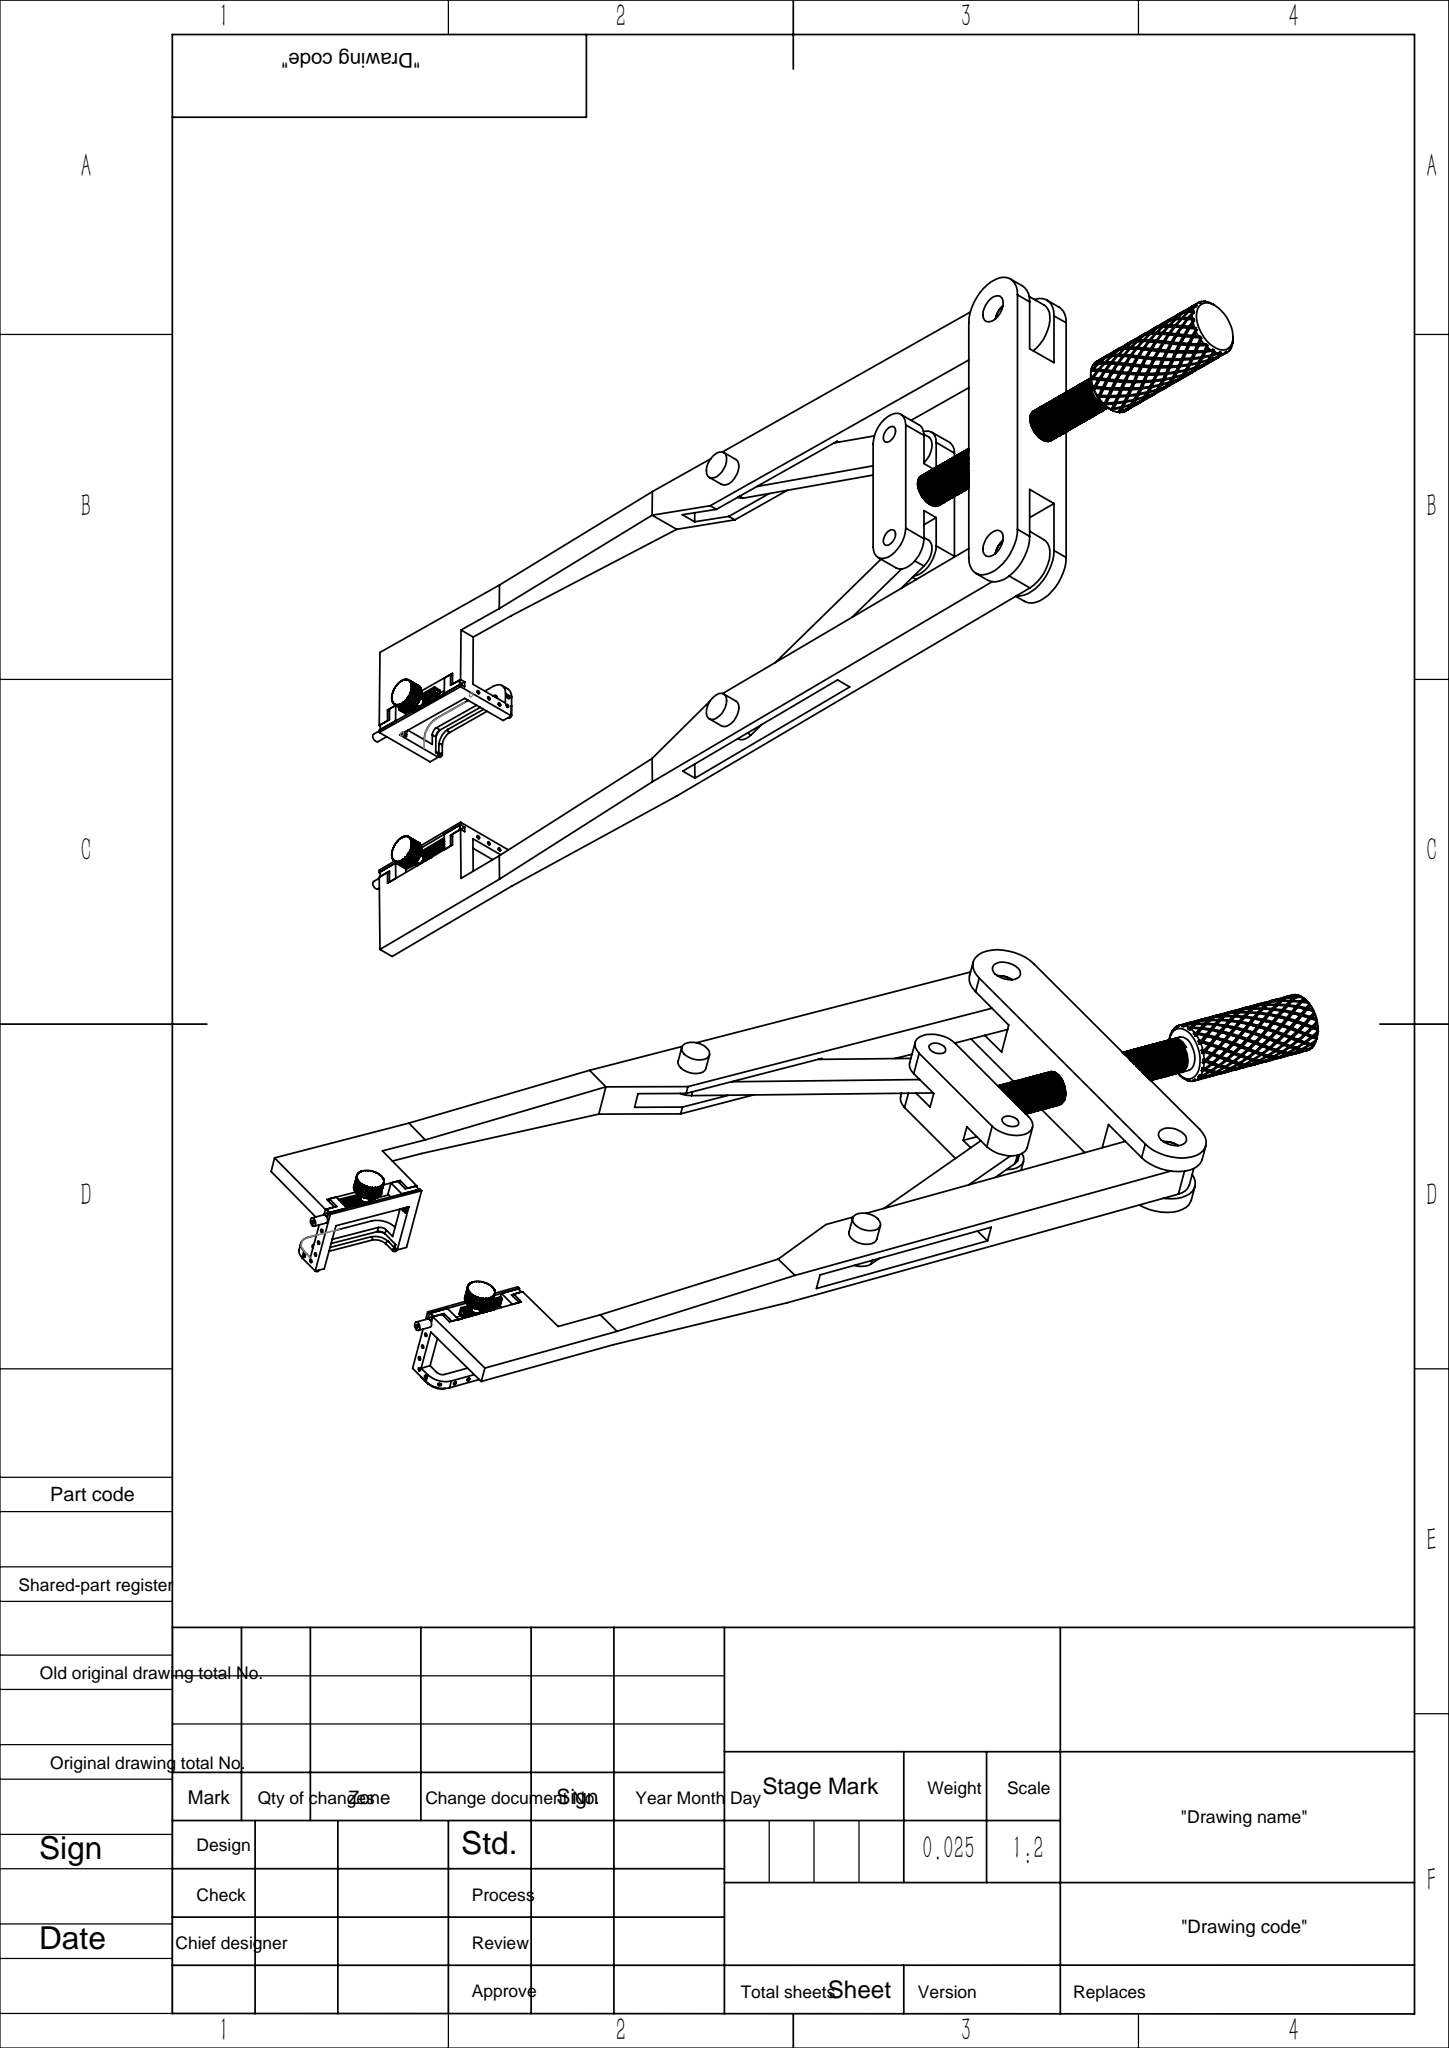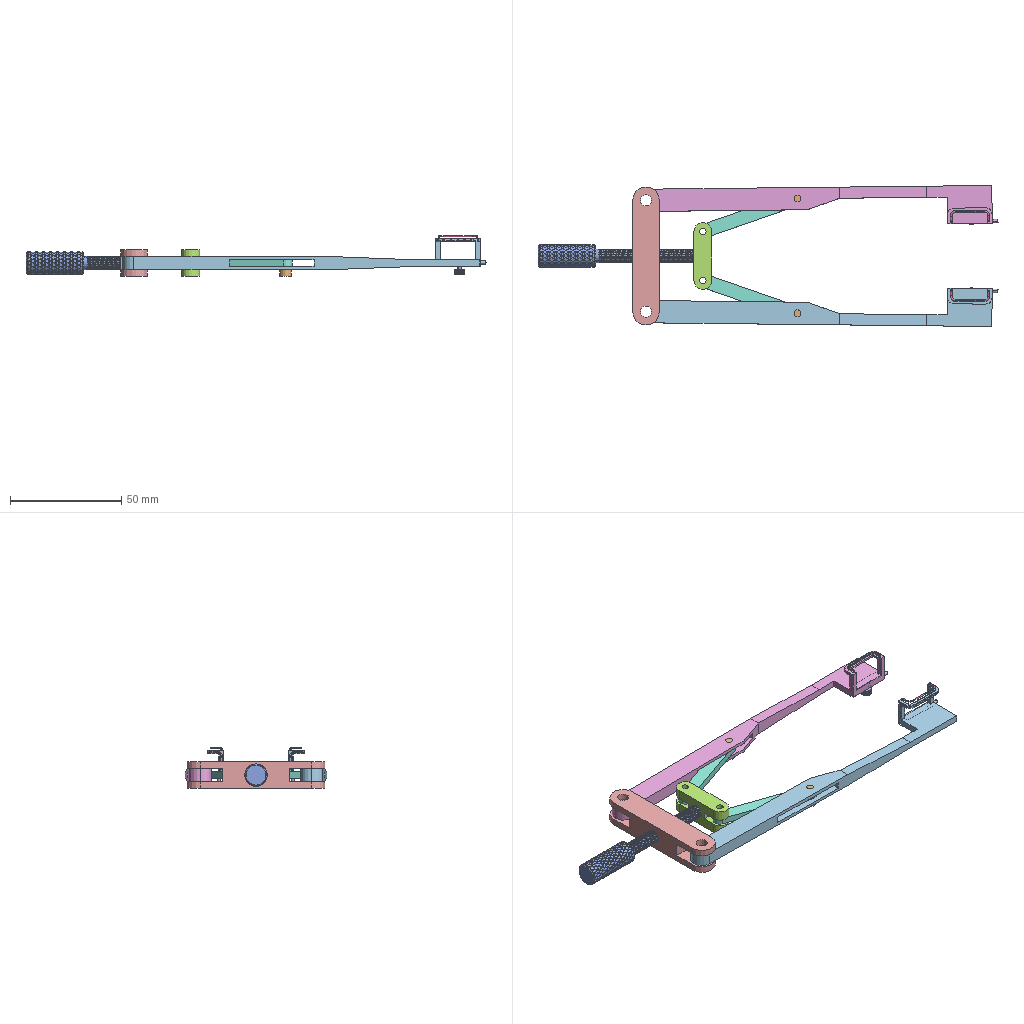Assembly | SolidWorks | 15 different items | 23 placed | box 207 x 63 x 18 mm
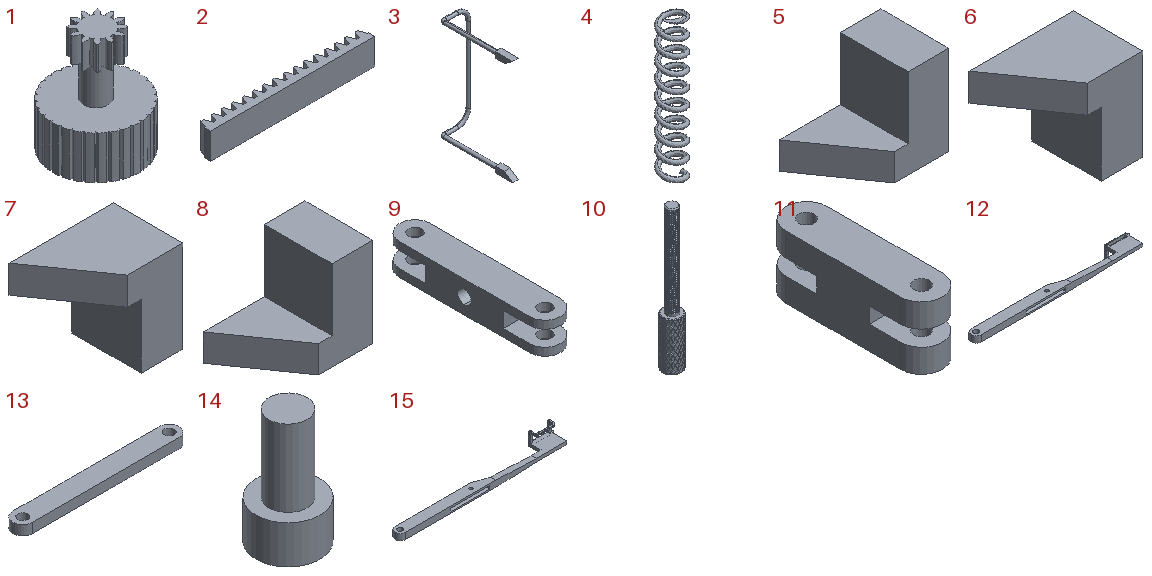Parts list (item | quantity | size | volume | features):
1 | x2 | 4.9 x 4.9 x 5.95 mm | 53.374 mm3 | features ICE 3, CirPattern 1, Extrusion 1, Scale 1
2 | x4 | 8.791 x 0.7439 x 1.4 mm | 6.578 mm3 | features Extrusion 1, ICE 1, Scale 1
3 | x2 | 5.2 x 12.8 x 18 mm | 16.656 mm3 | features 3DProfileFeature 2, ICE 2, Sweep 1
4 | x2 | 0.98 x 0.98 x 5.6 mm | 0.5935 mm3 | features ICE 2, Helix 1, Sweep 1
5 | x1 | 3.751 x 2.5 x 3.3 mm | 15.813 mm3 | features Extrusion 1, ICE 1
6 | x1 | 3.751 x 2.5 x 3.3 mm | 15.813 mm3 | features Extrusion 1, ICE 1
7 | x1 | 3.751 x 2.5 x 3.3 mm | 15.813 mm3 | features MirrorStock 1
8 | x1 | 3.751 x 2.5 x 3.3 mm | 15.813 mm3 | features MirrorStock 1
9 | x1 | 12 x 62 x 12 mm | 5967 mm3 | features ICE 2, 3DProfileFeature 1, Extrusion 1, HoleWzd 1
10 | x1 | 10 x 10.004 x 76 mm | 3336 mm3 | features Chamfer 1, CirPattern 1, Extrusion 1, ICE 1, MirrorPattern 1, SweepCut 1, SweepThread 1
11 | x1 | 8 x 30 x 12 mm | 2022 mm3 | features ICE 2, 3DProfileFeature 1, Extrusion 1, HoleWzd 1
12 | x1 | 162.952 x 17 x 14 mm | 5991 mm3 | features ICE 16, 3DProfileFeature 2, Chamfer 2, CurvePattern 1, Extrusion 1, MirrorPattern 1, SweepCut 1
13 | x2 | 51 x 6 x 3 mm | 852.412 mm3 | features Extrusion 1
14 | x2 | 5 x 5 x 9 mm | 101.316 mm3 | features Extrusion 1, ICE 1
15 | x1 | 162.952 x 17 x 14 mm | 5991 mm3 | features MirrorStock 1
Mates (type | each side: item.copy, entity, surface, feature):
Concentric | 9.1 face cylinder M6 Tapped Hole1 | 10.1 face cylinder Boss-Extrude2
Concentric | 10.1 face cylinder Boss-Extrude2 | 11.1 face cylinder M6 Tapped Hole1
Coincident | 10.1 face plane Boss-Extrude2 | 11.1 edge
Coincident | 9.1 face plane Boss-Extrude1 | 11.1 face plane Boss-Extrude1
Concentric | 9.1 face cylinder Cut-Extrude2 | 12.1 face cylinder Boss-Extrude1
Coincident | 9.1 face plane Cut-Extrude1 | 12.1 face plane Boss-Extrude1
Concentric | 11.1 face cylinder Cut-Extrude2 | 13.1 face cylinder Boss-Extrude1
Coincident | 11.1 face plane Cut-Extrude1 | 13.1 face plane Boss-Extrude1
Concentric | 12.1 face cylinder Boss-Extrude1 | 13.1 face cylinder Boss-Extrude1
Concentric | 12.1 face cylinder Boss-Extrude1 | 14.1 face cylinder Boss-Extrude2
Coincident | 12.1 face plane Boss-Extrude1 | 14.1 face plane Boss-Extrude1
Coincident | 1.1 face plane Boss-Extrude2 | 2.1 face plane Boss-Extrude1
DistanceDim | 1.1 face cylinder Boss-Extrude1 | 2.1 face plane Boss-Extrude1
Coincident | 12.1 face plane Cut-Extrude3 | 2.1 face plane Boss-Extrude1
DistanceDim | 2.1 face plane Boss-Extrude1 | 12.1 face plane Boss-Extrude2
DistanceDim | 1.1 face cylinder Boss-Extrude1 | 12.1 face plane Boss-Extrude2
Coincident | 2.1 face plane Boss-Extrude1 | 2.2 face plane Boss-Extrude1
Coincident | 12.1 face plane Cut-Extrude3 | 2.2 face plane Boss-Extrude1
Concentric | 12.1 face cylinder Cut-Extrude4 | 3.1 face cylinder Sweep1
DistanceDim | assembly plane | 9.1 face plane Cut-Extrude1
DistanceDim | 3.1 face cylinder Sweep1 | 12.1 face plane Boss-Extrude2
Coincident | 3.1 face plane Boss-Extrude1 | 4.1 face plane Cut-Extrude1
Concentric | 3.1 face cylinder Sweep1 | 4.1 select_type:24
Coincident | 3.1 face plane Boss-Extrude1 | 4.2 face plane Cut-Extrude1
Concentric | 3.1 face cylinder Sweep1 | 4.2 select_type:24
Coincident | 12.1 face plane Cut-Extrude3 | 5.1 face plane Boss-Extrude1
Coincident | 2.1 face plane Boss-Extrude1 | 5.1 face plane Boss-Extrude1
Coincident | 12.1 face plane Boss-Extrude2 | 5.1 face plane Boss-Extrude1
Coincident | 12.1 face plane Boss-Extrude2 | 6.1 face plane Boss-Extrude1
Coincident | 12.1 face plane Cut-Extrude3 | 6.1 face plane Boss-Extrude1
Coincident | 2.2 face plane Cut-Extrude1 | 6.1 face plane Boss-Extrude1
Coincident | 3.1 vertex | 6.1 face plane Boss-Extrude1
Coincident | 3.1 vertex | 5.1 face plane Boss-Extrude1
RackPinionDim | 2.1 edge | 1.1 face cylinder Boss-Extrude2